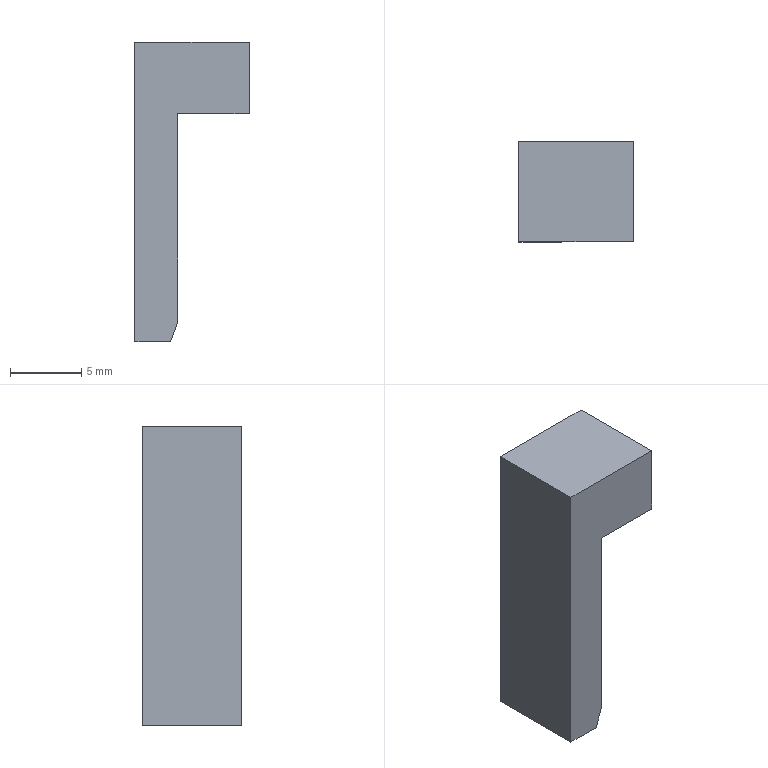Part | STEP file | D09 | 1 solid | 12 faces | box 8 x 7 x 21 mm | volume 572.033 mm3 | plane 10 | cylinder 2 | commonest cylinder face diameters 4.2 x2
STEP:
#1=CARTESIAN_POINT('',(0.,0.,0.));
#2=DIRECTION('',(0.,0.,1.));
#3=DIRECTION('',(1.,0.,0.));
#4=AXIS2_PLACEMENT_3D('',#1,#2,#3);
#5=CARTESIAN_POINT('',(1.9,-0.09279,19.));
#6=VERTEX_POINT('',#5);
#7=CARTESIAN_POINT('',(1.9,-0.09279,16.));
#8=VERTEX_POINT('',#7);
#9=CARTESIAN_POINT('',(1.9,-0.09279,19.));
#10=DIRECTION('',(0.,0.,-1.));
#11=VECTOR('',#10,1.);
#12=LINE('',#9,#11);
#13=CARTESIAN_POINT('',(4.,-0.09279,19.));
#14=DIRECTION('',(0.,0.,-1.));
#15=DIRECTION('',(-1.,0.,0.));
#16=AXIS2_PLACEMENT_3D('',#13,#14,#15);
#17=CYLINDRICAL_SURFACE('',#16,2.1);
#18=CARTESIAN_POINT('',(6.283,0.));
#19=DIRECTION('',(0.,1.));
#20=VECTOR('',#19,1.);
#21=LINE('',#18,#20);
#22=(GEOMETRIC_REPRESENTATION_CONTEXT(2)PARAMETRIC_REPRESENTATION_CONTEXT()REPRESENTATION_CONTEXT('',''));
#23=DEFINITIONAL_REPRESENTATION('',(#21),#22);
#24=PCURVE('',#17,#23);
#25=CARTESIAN_POINT('',(4.,-0.09279,19.));
#26=DIRECTION('',(0.,0.,-1.));
#27=DIRECTION('',(-1.,0.,0.));
#28=AXIS2_PLACEMENT_3D('',#25,#26,#27);
#29=CYLINDRICAL_SURFACE('',#28,2.1);
#30=CARTESIAN_POINT('',(0.,0.));
#31=DIRECTION('',(0.,1.));
#32=VECTOR('',#31,1.);
#33=LINE('',#30,#32);
#34=(GEOMETRIC_REPRESENTATION_CONTEXT(2)PARAMETRIC_REPRESENTATION_CONTEXT()REPRESENTATION_CONTEXT('',''));
#35=DEFINITIONAL_REPRESENTATION('',(#33),#34);
#36=PCURVE('',#29,#35);
#37=SURFACE_CURVE('',#12,(#24,#36),.PCURVE_S1.);
#38=EDGE_CURVE('',#6,#8,#37,.T.);
#39=ORIENTED_EDGE('',*,*,#38,.T.);
#40=CARTESIAN_POINT('',(6.1,-0.09279,16.));
#41=VERTEX_POINT('',#40);
#42=CARTESIAN_POINT('',(4.,-0.09279,16.));
#43=DIRECTION('',(0.,0.,-1.));
#44=DIRECTION('',(-1.,0.,0.));
#45=AXIS2_PLACEMENT_3D('',#42,#43,#44);
#46=CIRCLE('',#45,2.1);
#47=CARTESIAN_POINT('',(0.,3.));
#48=DIRECTION('',(1.,0.));
#49=VECTOR('',#48,1.);
#50=LINE('',#47,#49);
#51=(GEOMETRIC_REPRESENTATION_CONTEXT(2)PARAMETRIC_REPRESENTATION_CONTEXT()REPRESENTATION_CONTEXT('',''));
#52=DEFINITIONAL_REPRESENTATION('',(#50),#51);
#53=PCURVE('',#17,#52);
#54=CARTESIAN_POINT('',(0.,0.,16.));
#55=DIRECTION('',(0.,0.,-1.));
#56=DIRECTION('',(-1.,0.,0.));
#57=AXIS2_PLACEMENT_3D('',#54,#55,#56);
#58=PLANE('',#57);
#59=CARTESIAN_POINT('',(-4.,-0.09279));
#60=DIRECTION('',(1.,0.));
#61=AXIS2_PLACEMENT_2D('',#59,#60);
#62=CIRCLE('',#61,2.1);
#63=(GEOMETRIC_REPRESENTATION_CONTEXT(2)PARAMETRIC_REPRESENTATION_CONTEXT()REPRESENTATION_CONTEXT('',''));
#64=DEFINITIONAL_REPRESENTATION('',(#62),#63);
#65=PCURVE('',#58,#64);
#66=SURFACE_CURVE('',#46,(#53,#65),.PCURVE_S1.);
#67=EDGE_CURVE('',#41,#8,#66,.T.);
#68=ORIENTED_EDGE('',*,*,#67,.F.);
#69=CARTESIAN_POINT('',(6.1,-0.09279,19.));
#70=VERTEX_POINT('',#69);
#71=CARTESIAN_POINT('',(6.1,-0.09279,19.));
#72=DIRECTION('',(0.,0.,-1.));
#73=VECTOR('',#72,1.);
#74=LINE('',#71,#73);
#75=CARTESIAN_POINT('',(3.142,0.));
#76=DIRECTION('',(0.,1.));
#77=VECTOR('',#76,1.);
#78=LINE('',#75,#77);
#79=(GEOMETRIC_REPRESENTATION_CONTEXT(2)PARAMETRIC_REPRESENTATION_CONTEXT()REPRESENTATION_CONTEXT('',''));
#80=DEFINITIONAL_REPRESENTATION('',(#78),#79);
#81=PCURVE('',#17,#80);
#82=CARTESIAN_POINT('',(3.142,0.));
#83=DIRECTION('',(0.,1.));
#84=VECTOR('',#83,1.);
#85=LINE('',#82,#84);
#86=(GEOMETRIC_REPRESENTATION_CONTEXT(2)PARAMETRIC_REPRESENTATION_CONTEXT()REPRESENTATION_CONTEXT('',''));
#87=DEFINITIONAL_REPRESENTATION('',(#85),#86);
#88=PCURVE('',#29,#87);
#89=SURFACE_CURVE('',#74,(#81,#88),.PCURVE_S1.);
#90=EDGE_CURVE('',#70,#41,#89,.T.);
#91=ORIENTED_EDGE('',*,*,#90,.F.);
#92=CARTESIAN_POINT('',(4.,-0.09279,19.));
#93=DIRECTION('',(0.,0.,-1.));
#94=DIRECTION('',(-1.,0.,0.));
#95=AXIS2_PLACEMENT_3D('',#92,#93,#94);
#96=CIRCLE('',#95,2.1);
#97=CARTESIAN_POINT('',(0.,0.));
#98=DIRECTION('',(1.,0.));
#99=VECTOR('',#98,1.);
#100=LINE('',#97,#99);
#101=(GEOMETRIC_REPRESENTATION_CONTEXT(2)PARAMETRIC_REPRESENTATION_CONTEXT()REPRESENTATION_CONTEXT('',''));
#102=DEFINITIONAL_REPRESENTATION('',(#100),#101);
#103=PCURVE('',#17,#102);
#104=CARTESIAN_POINT('',(4.,-0.09279,19.));
#105=DIRECTION('',(0.,0.,-1.));
#106=DIRECTION('',(-1.,0.,0.));
#107=AXIS2_PLACEMENT_3D('',#104,#105,#106);
#108=PLANE('',#107);
#109=CARTESIAN_POINT('',(0.,0.));
#110=DIRECTION('',(1.,0.));
#111=AXIS2_PLACEMENT_2D('',#109,#110);
#112=CIRCLE('',#111,2.1);
#113=(GEOMETRIC_REPRESENTATION_CONTEXT(2)PARAMETRIC_REPRESENTATION_CONTEXT()REPRESENTATION_CONTEXT('',''));
#114=DEFINITIONAL_REPRESENTATION('',(#112),#113);
#115=PCURVE('',#108,#114);
#116=SURFACE_CURVE('',#96,(#103,#115),.PCURVE_S1.);
#117=EDGE_CURVE('',#70,#6,#116,.T.);
#118=ORIENTED_EDGE('',*,*,#117,.T.);
#119=EDGE_LOOP('',(#39,#68,#91,#118));
#120=FACE_BOUND('',#119,.F.);
#121=ADVANCED_FACE('',(#120),#17,.F.);
#122=CARTESIAN_POINT('',(1.5,-3.5,16.));
#123=VERTEX_POINT('',#122);
#124=CARTESIAN_POINT('',(1.5,-3.5,1.374));
#125=VERTEX_POINT('',#124);
#126=CARTESIAN_POINT('',(1.5,-3.5,16.));
#127=DIRECTION('',(0.,0.,-1.));
#128=VECTOR('',#127,1.);
#129=LINE('',#126,#128);
#130=CARTESIAN_POINT('',(1.5,3.5,16.));
#131=DIRECTION('',(-1.,0.,0.));
#132=DIRECTION('',(0.,-1.,0.));
#133=AXIS2_PLACEMENT_3D('',#130,#131,#132);
#134=PLANE('',#133);
#135=CARTESIAN_POINT('',(7.,0.));
#136=DIRECTION('',(0.,-1.));
#137=VECTOR('',#136,1.);
#138=LINE('',#135,#137);
#139=(GEOMETRIC_REPRESENTATION_CONTEXT(2)PARAMETRIC_REPRESENTATION_CONTEXT()REPRESENTATION_CONTEXT('',''));
#140=DEFINITIONAL_REPRESENTATION('',(#138),#139);
#141=PCURVE('',#134,#140);
#142=CARTESIAN_POINT('',(-1.5,-3.5,16.));
#143=DIRECTION('',(0.,1.,0.));
#144=DIRECTION('',(0.,0.,1.));
#145=AXIS2_PLACEMENT_3D('',#142,#143,#144);
#146=PLANE('',#145);
#147=CARTESIAN_POINT('',(0.,3.));
#148=DIRECTION('',(-1.,0.));
#149=VECTOR('',#148,1.);
#150=LINE('',#147,#149);
#151=(GEOMETRIC_REPRESENTATION_CONTEXT(2)PARAMETRIC_REPRESENTATION_CONTEXT()REPRESENTATION_CONTEXT('',''));
#152=DEFINITIONAL_REPRESENTATION('',(#150),#151);
#153=PCURVE('',#146,#152);
#154=SURFACE_CURVE('',#129,(#141,#153),.PCURVE_S1.);
#155=EDGE_CURVE('',#123,#125,#154,.T.);
#156=ORIENTED_EDGE('',*,*,#155,.T.);
#157=CARTESIAN_POINT('',(1.5,3.5,1.374));
#158=VERTEX_POINT('',#157);
#159=CARTESIAN_POINT('',(1.5,3.5,1.374));
#160=DIRECTION('',(0.,1.,0.));
#161=VECTOR('',#160,1.);
#162=LINE('',#159,#161);
#163=CARTESIAN_POINT('',(0.,-14.626));
#164=DIRECTION('',(-1.,0.));
#165=VECTOR('',#164,1.);
#166=LINE('',#163,#165);
#167=(GEOMETRIC_REPRESENTATION_CONTEXT(2)PARAMETRIC_REPRESENTATION_CONTEXT()REPRESENTATION_CONTEXT('',''));
#168=DEFINITIONAL_REPRESENTATION('',(#166),#167);
#169=PCURVE('',#134,#168);
#170=CARTESIAN_POINT('',(1.5,3.5,1.374));
#171=DIRECTION('',(-0.9397,0.,0.342));
#172=DIRECTION('',(0.,1.,0.));
#173=AXIS2_PLACEMENT_3D('',#170,#171,#172);
#174=PLANE('',#173);
#175=CARTESIAN_POINT('',(0.,0.));
#176=DIRECTION('',(1.,0.));
#177=VECTOR('',#176,1.);
#178=LINE('',#175,#177);
#179=(GEOMETRIC_REPRESENTATION_CONTEXT(2)PARAMETRIC_REPRESENTATION_CONTEXT()REPRESENTATION_CONTEXT('',''));
#180=DEFINITIONAL_REPRESENTATION('',(#178),#179);
#181=PCURVE('',#174,#180);
#182=SURFACE_CURVE('',#162,(#169,#181),.PCURVE_S1.);
#183=EDGE_CURVE('',#125,#158,#182,.T.);
#184=ORIENTED_EDGE('',*,*,#183,.T.);
#185=CARTESIAN_POINT('',(1.5,3.5,16.));
#186=VERTEX_POINT('',#185);
#187=CARTESIAN_POINT('',(1.5,3.5,16.));
#188=DIRECTION('',(0.,0.,-1.));
#189=VECTOR('',#188,1.);
#190=LINE('',#187,#189);
#191=CARTESIAN_POINT('',(0.,0.));
#192=DIRECTION('',(0.,-1.));
#193=VECTOR('',#192,1.);
#194=LINE('',#191,#193);
#195=(GEOMETRIC_REPRESENTATION_CONTEXT(2)PARAMETRIC_REPRESENTATION_CONTEXT()REPRESENTATION_CONTEXT('',''));
#196=DEFINITIONAL_REPRESENTATION('',(#194),#195);
#197=PCURVE('',#134,#196);
#198=CARTESIAN_POINT('',(-1.5,3.5,16.));
#199=DIRECTION('',(0.,-1.,0.));
#200=DIRECTION('',(0.,0.,-1.));
#201=AXIS2_PLACEMENT_3D('',#198,#199,#200);
#202=PLANE('',#201);
#203=CARTESIAN_POINT('',(0.,3.));
#204=DIRECTION('',(1.,0.));
#205=VECTOR('',#204,1.);
#206=LINE('',#203,#205);
#207=(GEOMETRIC_REPRESENTATION_CONTEXT(2)PARAMETRIC_REPRESENTATION_CONTEXT()REPRESENTATION_CONTEXT('',''));
#208=DEFINITIONAL_REPRESENTATION('',(#206),#207);
#209=PCURVE('',#202,#208);
#210=SURFACE_CURVE('',#190,(#197,#209),.PCURVE_S1.);
#211=EDGE_CURVE('',#186,#158,#210,.T.);
#212=ORIENTED_EDGE('',*,*,#211,.F.);
#213=CARTESIAN_POINT('',(1.5,3.5,16.));
#214=DIRECTION('',(0.,1.,0.));
#215=VECTOR('',#214,1.);
#216=LINE('',#213,#215);
#217=CARTESIAN_POINT('',(0.,0.));
#218=DIRECTION('',(-1.,0.));
#219=VECTOR('',#218,1.);
#220=LINE('',#217,#219);
#221=(GEOMETRIC_REPRESENTATION_CONTEXT(2)PARAMETRIC_REPRESENTATION_CONTEXT()REPRESENTATION_CONTEXT('',''));
#222=DEFINITIONAL_REPRESENTATION('',(#220),#221);
#223=PCURVE('',#134,#222);
#224=CARTESIAN_POINT('',(-1.5,3.5));
#225=DIRECTION('',(0.,1.));
#226=VECTOR('',#225,1.);
#227=LINE('',#224,#226);
#228=(GEOMETRIC_REPRESENTATION_CONTEXT(2)PARAMETRIC_REPRESENTATION_CONTEXT()REPRESENTATION_CONTEXT('',''));
#229=DEFINITIONAL_REPRESENTATION('',(#227),#228);
#230=PCURVE('',#58,#229);
#231=SURFACE_CURVE('',#216,(#223,#230),.PCURVE_S1.);
#232=EDGE_CURVE('',#123,#186,#231,.T.);
#233=ORIENTED_EDGE('',*,*,#232,.F.);
#234=EDGE_LOOP('',(#156,#184,#212,#233));
#235=FACE_BOUND('',#234,.T.);
#236=ADVANCED_FACE('',(#235),#134,.F.);
#237=ORIENTED_EDGE('',*,*,#211,.T.);
#238=CARTESIAN_POINT('',(1.,3.5,0.));
#239=VERTEX_POINT('',#238);
#240=CARTESIAN_POINT('',(1.5,3.5,1.374));
#241=DIRECTION('',(-0.342,0.,-0.9397));
#242=VECTOR('',#241,1.);
#243=LINE('',#240,#242);
#244=CARTESIAN_POINT('',(14.626,3.));
#245=DIRECTION('',(0.9397,-0.342));
#246=VECTOR('',#245,1.);
#247=LINE('',#244,#246);
#248=(GEOMETRIC_REPRESENTATION_CONTEXT(2)PARAMETRIC_REPRESENTATION_CONTEXT()REPRESENTATION_CONTEXT('',''));
#249=DEFINITIONAL_REPRESENTATION('',(#247),#248);
#250=PCURVE('',#202,#249);
#251=CARTESIAN_POINT('',(0.,0.));
#252=DIRECTION('',(0.,1.));
#253=VECTOR('',#252,1.);
#254=LINE('',#251,#253);
#255=(GEOMETRIC_REPRESENTATION_CONTEXT(2)PARAMETRIC_REPRESENTATION_CONTEXT()REPRESENTATION_CONTEXT('',''));
#256=DEFINITIONAL_REPRESENTATION('',(#254),#255);
#257=PCURVE('',#174,#256);
#258=SURFACE_CURVE('',#243,(#250,#257),.PCURVE_S1.);
#259=EDGE_CURVE('',#158,#239,#258,.T.);
#260=ORIENTED_EDGE('',*,*,#259,.T.);
#261=CARTESIAN_POINT('',(-1.5,3.5,0.));
#262=VERTEX_POINT('',#261);
#263=CARTESIAN_POINT('',(-1.5,3.5,0.));
#264=DIRECTION('',(-1.,0.,0.));
#265=VECTOR('',#264,1.);
#266=LINE('',#263,#265);
#267=CARTESIAN_POINT('',(16.,0.));
#268=DIRECTION('',(0.,-1.));
#269=VECTOR('',#268,1.);
#270=LINE('',#267,#269);
#271=(GEOMETRIC_REPRESENTATION_CONTEXT(2)PARAMETRIC_REPRESENTATION_CONTEXT()REPRESENTATION_CONTEXT('',''));
#272=DEFINITIONAL_REPRESENTATION('',(#270),#271);
#273=PCURVE('',#202,#272);
#274=CARTESIAN_POINT('',(0.,0.,0.));
#275=DIRECTION('',(0.,0.,1.));
#276=DIRECTION('',(1.,0.,0.));
#277=AXIS2_PLACEMENT_3D('',#274,#275,#276);
#278=PLANE('',#277);
#279=CARTESIAN_POINT('',(-1.5,3.5));
#280=DIRECTION('',(-1.,0.));
#281=VECTOR('',#280,1.);
#282=LINE('',#279,#281);
#283=(GEOMETRIC_REPRESENTATION_CONTEXT(2)PARAMETRIC_REPRESENTATION_CONTEXT()REPRESENTATION_CONTEXT('',''));
#284=DEFINITIONAL_REPRESENTATION('',(#282),#283);
#285=PCURVE('',#278,#284);
#286=SURFACE_CURVE('',#266,(#273,#285),.PCURVE_S1.);
#287=EDGE_CURVE('',#239,#262,#286,.T.);
#288=ORIENTED_EDGE('',*,*,#287,.T.);
#289=CARTESIAN_POINT('',(-1.5,3.5,21.));
#290=VERTEX_POINT('',#289);
#291=CARTESIAN_POINT('',(-1.5,3.5,16.));
#292=DIRECTION('',(0.,0.,-1.));
#293=VECTOR('',#292,1.);
#294=LINE('',#291,#293);
#295=CARTESIAN_POINT('',(0.,0.));
#296=DIRECTION('',(1.,0.));
#297=VECTOR('',#296,1.);
#298=LINE('',#295,#297);
#299=(GEOMETRIC_REPRESENTATION_CONTEXT(2)PARAMETRIC_REPRESENTATION_CONTEXT()REPRESENTATION_CONTEXT('',''));
#300=DEFINITIONAL_REPRESENTATION('',(#298),#299);
#301=PCURVE('',#202,#300);
#302=CARTESIAN_POINT('',(-1.5,3.5,16.));
#303=DIRECTION('',(1.,0.,0.));
#304=DIRECTION('',(0.,1.,0.));
#305=AXIS2_PLACEMENT_3D('',#302,#303,#304);
#306=PLANE('',#305);
#307=CARTESIAN_POINT('',(0.,0.));
#308=DIRECTION('',(0.,-1.));
#309=VECTOR('',#308,1.);
#310=LINE('',#307,#309);
#311=(GEOMETRIC_REPRESENTATION_CONTEXT(2)PARAMETRIC_REPRESENTATION_CONTEXT()REPRESENTATION_CONTEXT('',''));
#312=DEFINITIONAL_REPRESENTATION('',(#310),#311);
#313=PCURVE('',#306,#312);
#314=SURFACE_CURVE('',#294,(#301,#313),.PCURVE_S1.);
#315=EDGE_CURVE('',#290,#262,#314,.T.);
#316=ORIENTED_EDGE('',*,*,#315,.F.);
#317=CARTESIAN_POINT('',(6.5,3.5,21.));
#318=VERTEX_POINT('',#317);
#319=CARTESIAN_POINT('',(6.5,3.5,21.));
#320=DIRECTION('',(-1.,0.,0.));
#321=VECTOR('',#320,1.);
#322=LINE('',#319,#321);
#323=CARTESIAN_POINT('',(-5.,8.));
#324=DIRECTION('',(0.,-1.));
#325=VECTOR('',#324,1.);
#326=LINE('',#323,#325);
#327=(GEOMETRIC_REPRESENTATION_CONTEXT(2)PARAMETRIC_REPRESENTATION_CONTEXT()REPRESENTATION_CONTEXT('',''));
#328=DEFINITIONAL_REPRESENTATION('',(#326),#327);
#329=PCURVE('',#202,#328);
#330=CARTESIAN_POINT('',(0.,0.,21.));
#331=DIRECTION('',(0.,0.,-1.));
#332=DIRECTION('',(-1.,0.,0.));
#333=AXIS2_PLACEMENT_3D('',#330,#331,#332);
#334=PLANE('',#333);
#335=CARTESIAN_POINT('',(-6.5,3.5));
#336=DIRECTION('',(1.,0.));
#337=VECTOR('',#336,1.);
#338=LINE('',#335,#337);
#339=(GEOMETRIC_REPRESENTATION_CONTEXT(2)PARAMETRIC_REPRESENTATION_CONTEXT()REPRESENTATION_CONTEXT('',''));
#340=DEFINITIONAL_REPRESENTATION('',(#338),#339);
#341=PCURVE('',#334,#340);
#342=SURFACE_CURVE('',#322,(#329,#341),.PCURVE_S1.);
#343=EDGE_CURVE('',#318,#290,#342,.T.);
#344=ORIENTED_EDGE('',*,*,#343,.F.);
#345=CARTESIAN_POINT('',(6.5,3.5,16.));
#346=VERTEX_POINT('',#345);
#347=CARTESIAN_POINT('',(6.5,3.5,21.));
#348=DIRECTION('',(0.,0.,-1.));
#349=VECTOR('',#348,1.);
#350=LINE('',#347,#349);
#351=CARTESIAN_POINT('',(-5.,8.));
#352=DIRECTION('',(1.,0.));
#353=VECTOR('',#352,1.);
#354=LINE('',#351,#353);
#355=(GEOMETRIC_REPRESENTATION_CONTEXT(2)PARAMETRIC_REPRESENTATION_CONTEXT()REPRESENTATION_CONTEXT('',''));
#356=DEFINITIONAL_REPRESENTATION('',(#354),#355);
#357=PCURVE('',#202,#356);
#358=CARTESIAN_POINT('',(6.5,3.5,21.));
#359=DIRECTION('',(-1.,0.,0.));
#360=DIRECTION('',(0.,-1.,0.));
#361=AXIS2_PLACEMENT_3D('',#358,#359,#360);
#362=PLANE('',#361);
#363=CARTESIAN_POINT('',(0.,0.));
#364=DIRECTION('',(0.,-1.));
#365=VECTOR('',#364,1.);
#366=LINE('',#363,#365);
#367=(GEOMETRIC_REPRESENTATION_CONTEXT(2)PARAMETRIC_REPRESENTATION_CONTEXT()REPRESENTATION_CONTEXT('',''));
#368=DEFINITIONAL_REPRESENTATION('',(#366),#367);
#369=PCURVE('',#362,#368);
#370=SURFACE_CURVE('',#350,(#357,#369),.PCURVE_S1.);
#371=EDGE_CURVE('',#318,#346,#370,.T.);
#372=ORIENTED_EDGE('',*,*,#371,.T.);
#373=CARTESIAN_POINT('',(6.5,3.5,16.));
#374=DIRECTION('',(-1.,0.,0.));
#375=VECTOR('',#374,1.);
#376=LINE('',#373,#375);
#377=CARTESIAN_POINT('',(0.,8.));
#378=DIRECTION('',(0.,-1.));
#379=VECTOR('',#378,1.);
#380=LINE('',#377,#379);
#381=(GEOMETRIC_REPRESENTATION_CONTEXT(2)PARAMETRIC_REPRESENTATION_CONTEXT()REPRESENTATION_CONTEXT('',''));
#382=DEFINITIONAL_REPRESENTATION('',(#380),#381);
#383=PCURVE('',#202,#382);
#384=CARTESIAN_POINT('',(-6.5,3.5));
#385=DIRECTION('',(1.,0.));
#386=VECTOR('',#385,1.);
#387=LINE('',#384,#386);
#388=(GEOMETRIC_REPRESENTATION_CONTEXT(2)PARAMETRIC_REPRESENTATION_CONTEXT()REPRESENTATION_CONTEXT('',''));
#389=DEFINITIONAL_REPRESENTATION('',(#387),#388);
#390=PCURVE('',#58,#389);
#391=SURFACE_CURVE('',#376,(#383,#390),.PCURVE_S1.);
#392=EDGE_CURVE('',#346,#186,#391,.T.);
#393=ORIENTED_EDGE('',*,*,#392,.T.);
#394=EDGE_LOOP('',(#237,#260,#288,#316,#344,#372,#393));
#395=FACE_BOUND('',#394,.T.);
#396=ADVANCED_FACE('',(#395),#202,.F.);
#397=CARTESIAN_POINT('',(-1.5,-3.5,0.));
#398=VERTEX_POINT('',#397);
#399=CARTESIAN_POINT('',(-1.5,3.5,0.));
#400=DIRECTION('',(0.,-1.,0.));
#401=VECTOR('',#400,1.);
#402=LINE('',#399,#401);
#403=CARTESIAN_POINT('',(0.,-16.));
#404=DIRECTION('',(-1.,0.));
#405=VECTOR('',#404,1.);
#406=LINE('',#403,#405);
#407=(GEOMETRIC_REPRESENTATION_CONTEXT(2)PARAMETRIC_REPRESENTATION_CONTEXT()REPRESENTATION_CONTEXT('',''));
#408=DEFINITIONAL_REPRESENTATION('',(#406),#407);
#409=PCURVE('',#306,#408);
#410=CARTESIAN_POINT('',(-1.5,3.5));
#411=DIRECTION('',(0.,-1.));
#412=VECTOR('',#411,1.);
#413=LINE('',#410,#412);
#414=(GEOMETRIC_REPRESENTATION_CONTEXT(2)PARAMETRIC_REPRESENTATION_CONTEXT()REPRESENTATION_CONTEXT('',''));
#415=DEFINITIONAL_REPRESENTATION('',(#413),#414);
#416=PCURVE('',#278,#415);
#417=SURFACE_CURVE('',#402,(#409,#416),.PCURVE_S1.);
#418=EDGE_CURVE('',#262,#398,#417,.T.);
#419=ORIENTED_EDGE('',*,*,#418,.T.);
#420=CARTESIAN_POINT('',(-1.5,-3.5,21.));
#421=VERTEX_POINT('',#420);
#422=CARTESIAN_POINT('',(-1.5,-3.5,16.));
#423=DIRECTION('',(0.,0.,-1.));
#424=VECTOR('',#423,1.);
#425=LINE('',#422,#424);
#426=CARTESIAN_POINT('',(-7.,0.));
#427=DIRECTION('',(0.,-1.));
#428=VECTOR('',#427,1.);
#429=LINE('',#426,#428);
#430=(GEOMETRIC_REPRESENTATION_CONTEXT(2)PARAMETRIC_REPRESENTATION_CONTEXT()REPRESENTATION_CONTEXT('',''));
#431=DEFINITIONAL_REPRESENTATION('',(#429),#430);
#432=PCURVE('',#306,#431);
#433=CARTESIAN_POINT('',(0.,0.));
#434=DIRECTION('',(-1.,0.));
#435=VECTOR('',#434,1.);
#436=LINE('',#433,#435);
#437=(GEOMETRIC_REPRESENTATION_CONTEXT(2)PARAMETRIC_REPRESENTATION_CONTEXT()REPRESENTATION_CONTEXT('',''));
#438=DEFINITIONAL_REPRESENTATION('',(#436),#437);
#439=PCURVE('',#146,#438);
#440=SURFACE_CURVE('',#425,(#432,#439),.PCURVE_S1.);
#441=EDGE_CURVE('',#421,#398,#440,.T.);
#442=ORIENTED_EDGE('',*,*,#441,.F.);
#443=CARTESIAN_POINT('',(-1.5,3.5,21.));
#444=DIRECTION('',(0.,-1.,0.));
#445=VECTOR('',#444,1.);
#446=LINE('',#443,#445);
#447=CARTESIAN_POINT('',(0.,5.));
#448=DIRECTION('',(-1.,0.));
#449=VECTOR('',#448,1.);
#450=LINE('',#447,#449);
#451=(GEOMETRIC_REPRESENTATION_CONTEXT(2)PARAMETRIC_REPRESENTATION_CONTEXT()REPRESENTATION_CONTEXT('',''));
#452=DEFINITIONAL_REPRESENTATION('',(#450),#451);
#453=PCURVE('',#306,#452);
#454=CARTESIAN_POINT('',(1.5,3.5));
#455=DIRECTION('',(0.,-1.));
#456=VECTOR('',#455,1.);
#457=LINE('',#454,#456);
#458=(GEOMETRIC_REPRESENTATION_CONTEXT(2)PARAMETRIC_REPRESENTATION_CONTEXT()REPRESENTATION_CONTEXT('',''));
#459=DEFINITIONAL_REPRESENTATION('',(#457),#458);
#460=PCURVE('',#334,#459);
#461=SURFACE_CURVE('',#446,(#453,#460),.PCURVE_S1.);
#462=EDGE_CURVE('',#290,#421,#461,.T.);
#463=ORIENTED_EDGE('',*,*,#462,.F.);
#464=ORIENTED_EDGE('',*,*,#315,.T.);
#465=EDGE_LOOP('',(#419,#442,#463,#464));
#466=FACE_BOUND('',#465,.T.);
#467=ADVANCED_FACE('',(#466),#306,.F.);
#468=CARTESIAN_POINT('',(1.,-3.5,0.));
#469=VERTEX_POINT('',#468);
#470=CARTESIAN_POINT('',(-1.5,-3.5,0.));
#471=DIRECTION('',(1.,0.,0.));
#472=VECTOR('',#471,1.);
#473=LINE('',#470,#472);
#474=CARTESIAN_POINT('',(-16.,0.));
#475=DIRECTION('',(0.,1.));
#476=VECTOR('',#475,1.);
#477=LINE('',#474,#476);
#478=(GEOMETRIC_REPRESENTATION_CONTEXT(2)PARAMETRIC_REPRESENTATION_CONTEXT()REPRESENTATION_CONTEXT('',''));
#479=DEFINITIONAL_REPRESENTATION('',(#477),#478);
#480=PCURVE('',#146,#479);
#481=CARTESIAN_POINT('',(-1.5,-3.5));
#482=DIRECTION('',(1.,0.));
#483=VECTOR('',#482,1.);
#484=LINE('',#481,#483);
#485=(GEOMETRIC_REPRESENTATION_CONTEXT(2)PARAMETRIC_REPRESENTATION_CONTEXT()REPRESENTATION_CONTEXT('',''));
#486=DEFINITIONAL_REPRESENTATION('',(#484),#485);
#487=PCURVE('',#278,#486);
#488=SURFACE_CURVE('',#473,(#480,#487),.PCURVE_S1.);
#489=EDGE_CURVE('',#398,#469,#488,.T.);
#490=ORIENTED_EDGE('',*,*,#489,.T.);
#491=CARTESIAN_POINT('',(1.5,-3.5,1.374));
#492=DIRECTION('',(0.342,0.,0.9397));
#493=VECTOR('',#492,1.);
#494=LINE('',#491,#493);
#495=CARTESIAN_POINT('',(-14.626,3.));
#496=DIRECTION('',(0.9397,0.342));
#497=VECTOR('',#496,1.);
#498=LINE('',#495,#497);
#499=(GEOMETRIC_REPRESENTATION_CONTEXT(2)PARAMETRIC_REPRESENTATION_CONTEXT()REPRESENTATION_CONTEXT('',''));
#500=DEFINITIONAL_REPRESENTATION('',(#498),#499);
#501=PCURVE('',#146,#500);
#502=CARTESIAN_POINT('',(-7.,0.));
#503=DIRECTION('',(0.,-1.));
#504=VECTOR('',#503,1.);
#505=LINE('',#502,#504);
#506=(GEOMETRIC_REPRESENTATION_CONTEXT(2)PARAMETRIC_REPRESENTATION_CONTEXT()REPRESENTATION_CONTEXT('',''));
#507=DEFINITIONAL_REPRESENTATION('',(#505),#506);
#508=PCURVE('',#174,#507);
#509=SURFACE_CURVE('',#494,(#501,#508),.PCURVE_S1.);
#510=EDGE_CURVE('',#469,#125,#509,.T.);
#511=ORIENTED_EDGE('',*,*,#510,.T.);
#512=ORIENTED_EDGE('',*,*,#155,.F.);
#513=CARTESIAN_POINT('',(6.5,-3.5,16.));
#514=VERTEX_POINT('',#513);
#515=CARTESIAN_POINT('',(6.5,-3.5,16.));
#516=DIRECTION('',(1.,0.,0.));
#517=VECTOR('',#516,1.);
#518=LINE('',#515,#517);
#519=CARTESIAN_POINT('',(0.,8.));
#520=DIRECTION('',(0.,1.));
#521=VECTOR('',#520,1.);
#522=LINE('',#519,#521);
#523=(GEOMETRIC_REPRESENTATION_CONTEXT(2)PARAMETRIC_REPRESENTATION_CONTEXT()REPRESENTATION_CONTEXT('',''));
#524=DEFINITIONAL_REPRESENTATION('',(#522),#523);
#525=PCURVE('',#146,#524);
#526=CARTESIAN_POINT('',(-6.5,-3.5));
#527=DIRECTION('',(-1.,0.));
#528=VECTOR('',#527,1.);
#529=LINE('',#526,#528);
#530=(GEOMETRIC_REPRESENTATION_CONTEXT(2)PARAMETRIC_REPRESENTATION_CONTEXT()REPRESENTATION_CONTEXT('',''));
#531=DEFINITIONAL_REPRESENTATION('',(#529),#530);
#532=PCURVE('',#58,#531);
#533=SURFACE_CURVE('',#518,(#525,#532),.PCURVE_S1.);
#534=EDGE_CURVE('',#123,#514,#533,.T.);
#535=ORIENTED_EDGE('',*,*,#534,.T.);
#536=CARTESIAN_POINT('',(6.5,-3.5,21.));
#537=VERTEX_POINT('',#536);
#538=CARTESIAN_POINT('',(6.5,-3.5,21.));
#539=DIRECTION('',(0.,0.,-1.));
#540=VECTOR('',#539,1.);
#541=LINE('',#538,#540);
#542=CARTESIAN_POINT('',(5.,8.));
#543=DIRECTION('',(-1.,0.));
#544=VECTOR('',#543,1.);
#545=LINE('',#542,#544);
#546=(GEOMETRIC_REPRESENTATION_CONTEXT(2)PARAMETRIC_REPRESENTATION_CONTEXT()REPRESENTATION_CONTEXT('',''));
#547=DEFINITIONAL_REPRESENTATION('',(#545),#546);
#548=PCURVE('',#146,#547);
#549=CARTESIAN_POINT('',(7.,0.));
#550=DIRECTION('',(0.,-1.));
#551=VECTOR('',#550,1.);
#552=LINE('',#549,#551);
#553=(GEOMETRIC_REPRESENTATION_CONTEXT(2)PARAMETRIC_REPRESENTATION_CONTEXT()REPRESENTATION_CONTEXT('',''));
#554=DEFINITIONAL_REPRESENTATION('',(#552),#553);
#555=PCURVE('',#362,#554);
#556=SURFACE_CURVE('',#541,(#548,#555),.PCURVE_S1.);
#557=EDGE_CURVE('',#537,#514,#556,.T.);
#558=ORIENTED_EDGE('',*,*,#557,.F.);
#559=CARTESIAN_POINT('',(6.5,-3.5,21.));
#560=DIRECTION('',(1.,0.,0.));
#561=VECTOR('',#560,1.);
#562=LINE('',#559,#561);
#563=CARTESIAN_POINT('',(5.,8.));
#564=DIRECTION('',(0.,1.));
#565=VECTOR('',#564,1.);
#566=LINE('',#563,#565);
#567=(GEOMETRIC_REPRESENTATION_CONTEXT(2)PARAMETRIC_REPRESENTATION_CONTEXT()REPRESENTATION_CONTEXT('',''));
#568=DEFINITIONAL_REPRESENTATION('',(#566),#567);
#569=PCURVE('',#146,#568);
#570=CARTESIAN_POINT('',(-6.5,-3.5));
#571=DIRECTION('',(-1.,0.));
#572=VECTOR('',#571,1.);
#573=LINE('',#570,#572);
#574=(GEOMETRIC_REPRESENTATION_CONTEXT(2)PARAMETRIC_REPRESENTATION_CONTEXT()REPRESENTATION_CONTEXT('',''));
#575=DEFINITIONAL_REPRESENTATION('',(#573),#574);
#576=PCURVE('',#334,#575);
#577=SURFACE_CURVE('',#562,(#569,#576),.PCURVE_S1.);
#578=EDGE_CURVE('',#421,#537,#577,.T.);
#579=ORIENTED_EDGE('',*,*,#578,.F.);
#580=ORIENTED_EDGE('',*,*,#441,.T.);
#581=EDGE_LOOP('',(#490,#511,#512,#535,#558,#579,#580));
#582=FACE_BOUND('',#581,.T.);
#583=ADVANCED_FACE('',(#582),#146,.F.);
#584=ORIENTED_EDGE('',*,*,#287,.F.);
#585=CARTESIAN_POINT('',(1.,0.,0.));
#586=DIRECTION('',(0.,-1.,0.));
#587=VECTOR('',#586,1.);
#588=LINE('',#585,#587);
#589=CARTESIAN_POINT('',(1.,0.));
#590=DIRECTION('',(0.,-1.));
#591=VECTOR('',#590,1.);
#592=LINE('',#589,#591);
#593=(GEOMETRIC_REPRESENTATION_CONTEXT(2)PARAMETRIC_REPRESENTATION_CONTEXT()REPRESENTATION_CONTEXT('',''));
#594=DEFINITIONAL_REPRESENTATION('',(#592),#593);
#595=PCURVE('',#278,#594);
#596=CARTESIAN_POINT('',(-3.5,1.462));
#597=DIRECTION('',(-1.,0.));
#598=VECTOR('',#597,1.);
#599=LINE('',#596,#598);
#600=(GEOMETRIC_REPRESENTATION_CONTEXT(2)PARAMETRIC_REPRESENTATION_CONTEXT()REPRESENTATION_CONTEXT('',''));
#601=DEFINITIONAL_REPRESENTATION('',(#599),#600);
#602=PCURVE('',#174,#601);
#603=SURFACE_CURVE('',#588,(#595,#602),.PCURVE_S1.);
#604=EDGE_CURVE('',#239,#469,#603,.T.);
#605=ORIENTED_EDGE('',*,*,#604,.T.);
#606=ORIENTED_EDGE('',*,*,#489,.F.);
#607=ORIENTED_EDGE('',*,*,#418,.F.);
#608=EDGE_LOOP('',(#584,#605,#606,#607));
#609=FACE_BOUND('',#608,.T.);
#610=ADVANCED_FACE('',(#609),#278,.F.);
#611=CARTESIAN_POINT('',(6.5,3.5,16.));
#612=DIRECTION('',(0.,1.,0.));
#613=VECTOR('',#612,1.);
#614=LINE('',#611,#613);
#615=CARTESIAN_POINT('',(0.,-5.));
#616=DIRECTION('',(-1.,0.));
#617=VECTOR('',#616,1.);
#618=LINE('',#615,#617);
#619=(GEOMETRIC_REPRESENTATION_CONTEXT(2)PARAMETRIC_REPRESENTATION_CONTEXT()REPRESENTATION_CONTEXT('',''));
#620=DEFINITIONAL_REPRESENTATION('',(#618),#619);
#621=PCURVE('',#362,#620);
#622=CARTESIAN_POINT('',(-6.5,3.5));
#623=DIRECTION('',(0.,1.));
#624=VECTOR('',#623,1.);
#625=LINE('',#622,#624);
#626=(GEOMETRIC_REPRESENTATION_CONTEXT(2)PARAMETRIC_REPRESENTATION_CONTEXT()REPRESENTATION_CONTEXT('',''));
#627=DEFINITIONAL_REPRESENTATION('',(#625),#626);
#628=PCURVE('',#58,#627);
#629=SURFACE_CURVE('',#614,(#621,#628),.PCURVE_S1.);
#630=EDGE_CURVE('',#514,#346,#629,.T.);
#631=ORIENTED_EDGE('',*,*,#630,.T.);
#632=ORIENTED_EDGE('',*,*,#371,.F.);
#633=CARTESIAN_POINT('',(6.5,3.5,21.));
#634=DIRECTION('',(0.,1.,0.));
#635=VECTOR('',#634,1.);
#636=LINE('',#633,#635);
#637=CARTESIAN_POINT('',(0.,0.));
#638=DIRECTION('',(-1.,0.));
#639=VECTOR('',#638,1.);
#640=LINE('',#637,#639);
#641=(GEOMETRIC_REPRESENTATION_CONTEXT(2)PARAMETRIC_REPRESENTATION_CONTEXT()REPRESENTATION_CONTEXT('',''));
#642=DEFINITIONAL_REPRESENTATION('',(#640),#641);
#643=PCURVE('',#362,#642);
#644=CARTESIAN_POINT('',(-6.5,3.5));
#645=DIRECTION('',(0.,1.));
#646=VECTOR('',#645,1.);
#647=LINE('',#644,#646);
#648=(GEOMETRIC_REPRESENTATION_CONTEXT(2)PARAMETRIC_REPRESENTATION_CONTEXT()REPRESENTATION_CONTEXT('',''));
#649=DEFINITIONAL_REPRESENTATION('',(#647),#648);
#650=PCURVE('',#334,#649);
#651=SURFACE_CURVE('',#636,(#643,#650),.PCURVE_S1.);
#652=EDGE_CURVE('',#537,#318,#651,.T.);
#653=ORIENTED_EDGE('',*,*,#652,.F.);
#654=ORIENTED_EDGE('',*,*,#557,.T.);
#655=EDGE_LOOP('',(#631,#632,#653,#654));
#656=FACE_BOUND('',#655,.T.);
#657=ADVANCED_FACE('',(#656),#362,.F.);
#658=ORIENTED_EDGE('',*,*,#652,.T.);
#659=ORIENTED_EDGE('',*,*,#343,.T.);
#660=ORIENTED_EDGE('',*,*,#462,.T.);
#661=ORIENTED_EDGE('',*,*,#578,.T.);
#662=EDGE_LOOP('',(#658,#659,#660,#661));
#663=FACE_BOUND('',#662,.T.);
#664=ADVANCED_FACE('',(#663),#334,.F.);
#665=CARTESIAN_POINT('',(4.,-0.09279,16.));
#666=DIRECTION('',(0.,0.,-1.));
#667=DIRECTION('',(-1.,0.,0.));
#668=AXIS2_PLACEMENT_3D('',#665,#666,#667);
#669=CIRCLE('',#668,2.1);
#670=CARTESIAN_POINT('',(-4.,-0.09279));
#671=DIRECTION('',(1.,0.));
#672=AXIS2_PLACEMENT_2D('',#670,#671);
#673=CIRCLE('',#672,2.1);
#674=(GEOMETRIC_REPRESENTATION_CONTEXT(2)PARAMETRIC_REPRESENTATION_CONTEXT()REPRESENTATION_CONTEXT('',''));
#675=DEFINITIONAL_REPRESENTATION('',(#673),#674);
#676=PCURVE('',#58,#675);
#677=CARTESIAN_POINT('',(0.,3.));
#678=DIRECTION('',(1.,0.));
#679=VECTOR('',#678,1.);
#680=LINE('',#677,#679);
#681=(GEOMETRIC_REPRESENTATION_CONTEXT(2)PARAMETRIC_REPRESENTATION_CONTEXT()REPRESENTATION_CONTEXT('',''));
#682=DEFINITIONAL_REPRESENTATION('',(#680),#681);
#683=PCURVE('',#29,#682);
#684=SURFACE_CURVE('',#669,(#676,#683),.PCURVE_S1.);
#685=EDGE_CURVE('',#8,#41,#684,.T.);
#686=ORIENTED_EDGE('',*,*,#685,.F.);
#687=ORIENTED_EDGE('',*,*,#67,.F.);
#688=EDGE_LOOP('',(#686,#687));
#689=FACE_BOUND('',#688,.T.);
#690=ORIENTED_EDGE('',*,*,#534,.F.);
#691=ORIENTED_EDGE('',*,*,#232,.T.);
#692=ORIENTED_EDGE('',*,*,#392,.F.);
#693=ORIENTED_EDGE('',*,*,#630,.F.);
#694=EDGE_LOOP('',(#690,#691,#692,#693));
#695=FACE_BOUND('',#694,.T.);
#696=ADVANCED_FACE('',(#689,#695),#58,.T.);
#697=ORIENTED_EDGE('',*,*,#685,.F.);
#698=ORIENTED_EDGE('',*,*,#38,.F.);
#699=CARTESIAN_POINT('',(4.,-0.09279,19.));
#700=DIRECTION('',(0.,0.,-1.));
#701=DIRECTION('',(-1.,0.,0.));
#702=AXIS2_PLACEMENT_3D('',#699,#700,#701);
#703=CIRCLE('',#702,2.1);
#704=CARTESIAN_POINT('',(0.,0.));
#705=DIRECTION('',(1.,0.));
#706=VECTOR('',#705,1.);
#707=LINE('',#704,#706);
#708=(GEOMETRIC_REPRESENTATION_CONTEXT(2)PARAMETRIC_REPRESENTATION_CONTEXT()REPRESENTATION_CONTEXT('',''));
#709=DEFINITIONAL_REPRESENTATION('',(#707),#708);
#710=PCURVE('',#29,#709);
#711=CARTESIAN_POINT('',(0.,0.));
#712=DIRECTION('',(1.,0.));
#713=AXIS2_PLACEMENT_2D('',#711,#712);
#714=CIRCLE('',#713,2.1);
#715=(GEOMETRIC_REPRESENTATION_CONTEXT(2)PARAMETRIC_REPRESENTATION_CONTEXT()REPRESENTATION_CONTEXT('',''));
#716=DEFINITIONAL_REPRESENTATION('',(#714),#715);
#717=PCURVE('',#108,#716);
#718=SURFACE_CURVE('',#703,(#710,#717),.PCURVE_S1.);
#719=EDGE_CURVE('',#6,#70,#718,.T.);
#720=ORIENTED_EDGE('',*,*,#719,.T.);
#721=ORIENTED_EDGE('',*,*,#90,.T.);
#722=EDGE_LOOP('',(#697,#698,#720,#721));
#723=FACE_BOUND('',#722,.F.);
#724=ADVANCED_FACE('',(#723),#29,.F.);
#725=ORIENTED_EDGE('',*,*,#719,.T.);
#726=ORIENTED_EDGE('',*,*,#117,.T.);
#727=EDGE_LOOP('',(#725,#726));
#728=FACE_BOUND('',#727,.T.);
#729=ADVANCED_FACE('',(#728),#108,.T.);
#730=ORIENTED_EDGE('',*,*,#510,.F.);
#731=ORIENTED_EDGE('',*,*,#604,.F.);
#732=ORIENTED_EDGE('',*,*,#259,.F.);
#733=ORIENTED_EDGE('',*,*,#183,.F.);
#734=EDGE_LOOP('',(#730,#731,#732,#733));
#735=FACE_BOUND('',#734,.T.);
#736=ADVANCED_FACE('',(#735),#174,.F.);
#737=CLOSED_SHELL('',(#121,#236,#396,#467,#583,#610,#657,#664,#696,#724,#729,#736));
#738=MANIFOLD_SOLID_BREP('',#737);
#739=(LENGTH_UNIT()NAMED_UNIT(*)SI_UNIT(.MILLI.,.METRE.));
#740=UNCERTAINTY_MEASURE_WITH_UNIT(LENGTH_MEASURE(0.0000001),#739,'','');
#741=(NAMED_UNIT(*)PLANE_ANGLE_UNIT()SI_UNIT($,.RADIAN.));
#742=(NAMED_UNIT(*)SI_UNIT($,.STERADIAN.)SOLID_ANGLE_UNIT());
#743=(GEOMETRIC_REPRESENTATION_CONTEXT(3)GLOBAL_UNCERTAINTY_ASSIGNED_CONTEXT((#740))GLOBAL_UNIT_ASSIGNED_CONTEXT((#739,#741,#742))REPRESENTATION_CONTEXT('',''));
#744=ADVANCED_BREP_SHAPE_REPRESENTATION('',(#4,#738),#743);